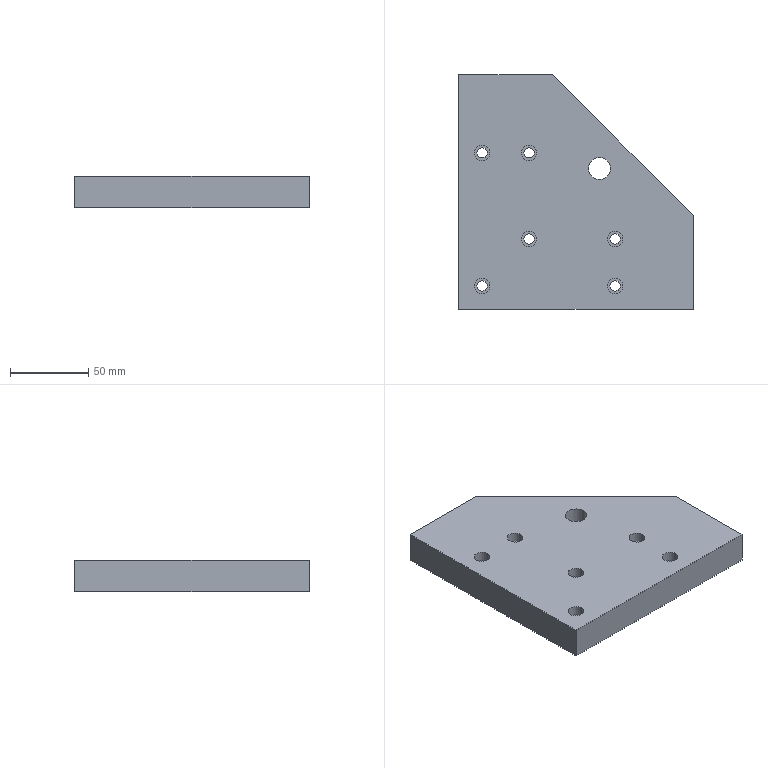Part | STEP file | PN_0022 Foot fixing plate | 1 solid | 39 faces | box 150 x 150 x 20 mm | volume 360114 mm3 | cylinder 26 | plane 13 | commonest cylinder face diameters 6.6 x12 10 x12 14 x2